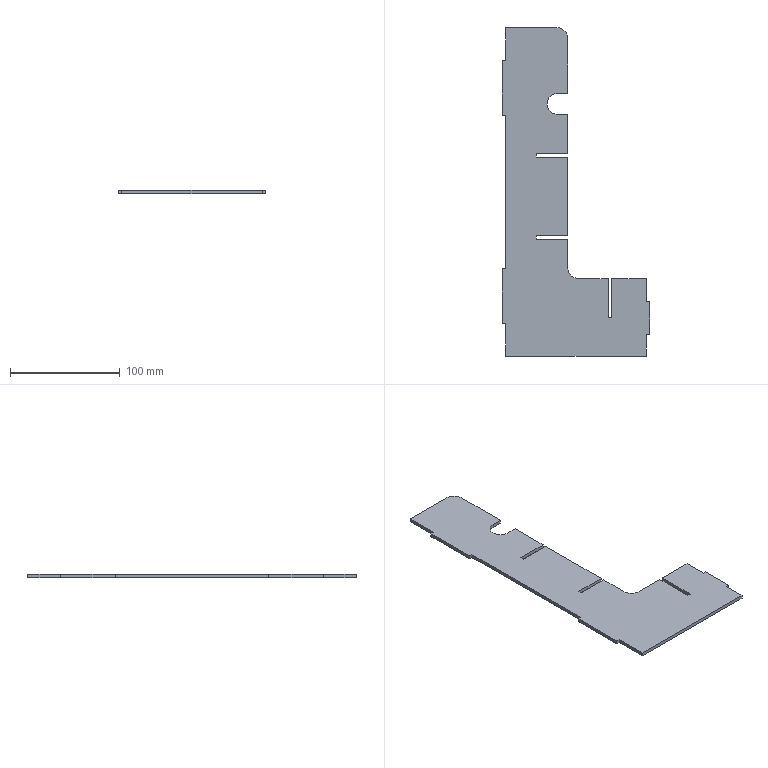Part | SolidWorks | features FlatPattern 1, SMBaseFlange 1, SheetMetal 1 | 1 solid | 38 faces | box 134.6 x 300 x 3.2 mm | volume 70099 mm3 | plane 35 | cylinder 3 | commonest cylinder face diameters 20 x2 19 x1
STEP:
#1=CARTESIAN_POINT('',(0.,-9.5,0.));
#2=VERTEX_POINT('',#1);
#3=CARTESIAN_POINT('',(0.,9.5,0.));
#4=VERTEX_POINT('',#3);
#5=CARTESIAN_POINT('',(0.,0.,0.));
#6=DIRECTION('',(0.,0.,-1.));
#7=DIRECTION('',(1.,0.,0.));
#8=AXIS2_PLACEMENT_3D('',#5,#6,#7);
#9=CIRCLE('',#8,9.5);
#10=EDGE_CURVE('',#2,#4,#9,.T.);
#11=ORIENTED_EDGE('',*,*,#10,.F.);
#12=CARTESIAN_POINT('',(0.,-9.5,-3.2));
#13=VERTEX_POINT('',#12);
#14=CARTESIAN_POINT('',(0.,-9.5,-3.2));
#15=DIRECTION('',(0.,0.,1.));
#16=VECTOR('',#15,1000.);
#17=LINE('',#14,#16);
#18=EDGE_CURVE('',#13,#2,#17,.T.);
#19=ORIENTED_EDGE('',*,*,#18,.F.);
#20=CARTESIAN_POINT('',(0.,9.5,-3.2));
#21=VERTEX_POINT('',#20);
#22=CARTESIAN_POINT('',(0.,0.,-3.2));
#23=DIRECTION('',(0.,0.,-1.));
#24=DIRECTION('',(1.,0.,0.));
#25=AXIS2_PLACEMENT_3D('',#22,#23,#24);
#26=CIRCLE('',#25,9.5);
#27=EDGE_CURVE('',#13,#21,#26,.T.);
#28=ORIENTED_EDGE('',*,*,#27,.T.);
#29=CARTESIAN_POINT('',(0.,9.5,-3.2));
#30=DIRECTION('',(0.,0.,1.));
#31=VECTOR('',#30,1000.);
#32=LINE('',#29,#31);
#33=EDGE_CURVE('',#21,#4,#32,.T.);
#34=ORIENTED_EDGE('',*,*,#33,.T.);
#35=EDGE_LOOP('',(#11,#19,#28,#34));
#36=FACE_OUTER_BOUND('',#35,.T.);
#37=CARTESIAN_POINT('',(0.,0.,-3.2));
#38=DIRECTION('',(0.,0.,1.));
#39=DIRECTION('',(1.,0.,0.));
#40=AXIS2_PLACEMENT_3D('',#37,#38,#39);
#41=CYLINDRICAL_SURFACE('',#40,9.5);
#42=ADVANCED_FACE('',(#36),#41,.F.);
#43=CARTESIAN_POINT('',(9.5,-9.5,0.));
#44=VERTEX_POINT('',#43);
#45=CARTESIAN_POINT('',(0.,-9.5,0.));
#46=DIRECTION('',(-1.,0.,0.));
#47=VECTOR('',#46,1000.);
#48=LINE('',#45,#47);
#49=EDGE_CURVE('',#44,#2,#48,.T.);
#50=ORIENTED_EDGE('',*,*,#49,.F.);
#51=CARTESIAN_POINT('',(9.5,-9.5,-3.2));
#52=VERTEX_POINT('',#51);
#53=CARTESIAN_POINT('',(9.5,-9.5,-3.2));
#54=DIRECTION('',(0.,0.,1.));
#55=VECTOR('',#54,1000.);
#56=LINE('',#53,#55);
#57=EDGE_CURVE('',#52,#44,#56,.T.);
#58=ORIENTED_EDGE('',*,*,#57,.F.);
#59=CARTESIAN_POINT('',(0.,-9.5,-3.2));
#60=DIRECTION('',(-1.,0.,0.));
#61=VECTOR('',#60,1000.);
#62=LINE('',#59,#61);
#63=EDGE_CURVE('',#52,#13,#62,.T.);
#64=ORIENTED_EDGE('',*,*,#63,.T.);
#65=ORIENTED_EDGE('',*,*,#18,.T.);
#66=EDGE_LOOP('',(#50,#58,#64,#65));
#67=FACE_OUTER_BOUND('',#66,.T.);
#68=CARTESIAN_POINT('',(0.,-9.5,-3.2));
#69=DIRECTION('',(0.,1.,0.));
#70=DIRECTION('',(0.,0.,1.));
#71=AXIS2_PLACEMENT_3D('',#68,#69,#70);
#72=PLANE('',#71);
#73=ADVANCED_FACE('',(#67),#72,.T.);
#74=CARTESIAN_POINT('',(9.5,-45.5,0.));
#75=VERTEX_POINT('',#74);
#76=CARTESIAN_POINT('',(9.5,-9.5,0.));
#77=DIRECTION('',(0.,1.,0.));
#78=VECTOR('',#77,1000.);
#79=LINE('',#76,#78);
#80=EDGE_CURVE('',#75,#44,#79,.T.);
#81=ORIENTED_EDGE('',*,*,#80,.F.);
#82=CARTESIAN_POINT('',(9.5,-45.5,-3.2));
#83=VERTEX_POINT('',#82);
#84=CARTESIAN_POINT('',(9.5,-45.5,-3.2));
#85=DIRECTION('',(0.,0.,1.));
#86=VECTOR('',#85,1000.);
#87=LINE('',#84,#86);
#88=EDGE_CURVE('',#83,#75,#87,.T.);
#89=ORIENTED_EDGE('',*,*,#88,.F.);
#90=CARTESIAN_POINT('',(9.5,-9.5,-3.2));
#91=DIRECTION('',(0.,1.,0.));
#92=VECTOR('',#91,1000.);
#93=LINE('',#90,#92);
#94=EDGE_CURVE('',#83,#52,#93,.T.);
#95=ORIENTED_EDGE('',*,*,#94,.T.);
#96=ORIENTED_EDGE('',*,*,#57,.T.);
#97=EDGE_LOOP('',(#81,#89,#95,#96));
#98=FACE_OUTER_BOUND('',#97,.T.);
#99=CARTESIAN_POINT('',(9.5,-9.5,-3.2));
#100=DIRECTION('',(1.,0.,0.));
#101=DIRECTION('',(0.,1.,0.));
#102=AXIS2_PLACEMENT_3D('',#99,#100,#101);
#103=PLANE('',#102);
#104=ADVANCED_FACE('',(#98),#103,.T.);
#105=CARTESIAN_POINT('',(-19.3,-45.5,0.));
#106=VERTEX_POINT('',#105);
#107=CARTESIAN_POINT('',(9.5,-45.5,0.));
#108=DIRECTION('',(1.,0.,0.));
#109=VECTOR('',#108,1000.);
#110=LINE('',#107,#109);
#111=EDGE_CURVE('',#106,#75,#110,.T.);
#112=ORIENTED_EDGE('',*,*,#111,.F.);
#113=CARTESIAN_POINT('',(-19.3,-45.5,-3.2));
#114=VERTEX_POINT('',#113);
#115=CARTESIAN_POINT('',(-19.3,-45.5,-3.2));
#116=DIRECTION('',(0.,0.,1.));
#117=VECTOR('',#116,1000.);
#118=LINE('',#115,#117);
#119=EDGE_CURVE('',#114,#106,#118,.T.);
#120=ORIENTED_EDGE('',*,*,#119,.F.);
#121=CARTESIAN_POINT('',(9.5,-45.5,-3.2));
#122=DIRECTION('',(1.,0.,0.));
#123=VECTOR('',#122,1000.);
#124=LINE('',#121,#123);
#125=EDGE_CURVE('',#114,#83,#124,.T.);
#126=ORIENTED_EDGE('',*,*,#125,.T.);
#127=ORIENTED_EDGE('',*,*,#88,.T.);
#128=EDGE_LOOP('',(#112,#120,#126,#127));
#129=FACE_OUTER_BOUND('',#128,.T.);
#130=CARTESIAN_POINT('',(9.5,-45.5,-3.2));
#131=DIRECTION('',(0.,-1.,0.));
#132=DIRECTION('',(0.,0.,-1.));
#133=AXIS2_PLACEMENT_3D('',#130,#131,#132);
#134=PLANE('',#133);
#135=ADVANCED_FACE('',(#129),#134,.T.);
#136=CARTESIAN_POINT('',(-19.3,-48.7,0.));
#137=VERTEX_POINT('',#136);
#138=CARTESIAN_POINT('',(-19.3,-45.5,0.));
#139=DIRECTION('',(0.,1.,0.));
#140=VECTOR('',#139,1000.);
#141=LINE('',#138,#140);
#142=EDGE_CURVE('',#137,#106,#141,.T.);
#143=ORIENTED_EDGE('',*,*,#142,.F.);
#144=CARTESIAN_POINT('',(-19.3,-48.7,-3.2));
#145=VERTEX_POINT('',#144);
#146=CARTESIAN_POINT('',(-19.3,-48.7,-3.2));
#147=DIRECTION('',(0.,0.,1.));
#148=VECTOR('',#147,1000.);
#149=LINE('',#146,#148);
#150=EDGE_CURVE('',#145,#137,#149,.T.);
#151=ORIENTED_EDGE('',*,*,#150,.F.);
#152=CARTESIAN_POINT('',(-19.3,-45.5,-3.2));
#153=DIRECTION('',(0.,1.,0.));
#154=VECTOR('',#153,1000.);
#155=LINE('',#152,#154);
#156=EDGE_CURVE('',#145,#114,#155,.T.);
#157=ORIENTED_EDGE('',*,*,#156,.T.);
#158=ORIENTED_EDGE('',*,*,#119,.T.);
#159=EDGE_LOOP('',(#143,#151,#157,#158));
#160=FACE_OUTER_BOUND('',#159,.T.);
#161=CARTESIAN_POINT('',(-19.3,-45.5,-3.2));
#162=DIRECTION('',(1.,0.,0.));
#163=DIRECTION('',(0.,0.,-1.));
#164=AXIS2_PLACEMENT_3D('',#161,#162,#163);
#165=PLANE('',#164);
#166=ADVANCED_FACE('',(#160),#165,.T.);
#167=CARTESIAN_POINT('',(9.5,-48.7,0.));
#168=VERTEX_POINT('',#167);
#169=CARTESIAN_POINT('',(-19.3,-48.7,0.));
#170=DIRECTION('',(-1.,0.,0.));
#171=VECTOR('',#170,1000.);
#172=LINE('',#169,#171);
#173=EDGE_CURVE('',#168,#137,#172,.T.);
#174=ORIENTED_EDGE('',*,*,#173,.F.);
#175=CARTESIAN_POINT('',(9.5,-48.7,-3.2));
#176=VERTEX_POINT('',#175);
#177=CARTESIAN_POINT('',(9.5,-48.7,-3.2));
#178=DIRECTION('',(0.,0.,1.));
#179=VECTOR('',#178,1000.);
#180=LINE('',#177,#179);
#181=EDGE_CURVE('',#176,#168,#180,.T.);
#182=ORIENTED_EDGE('',*,*,#181,.F.);
#183=CARTESIAN_POINT('',(-19.3,-48.7,-3.2));
#184=DIRECTION('',(-1.,0.,0.));
#185=VECTOR('',#184,1000.);
#186=LINE('',#183,#185);
#187=EDGE_CURVE('',#176,#145,#186,.T.);
#188=ORIENTED_EDGE('',*,*,#187,.T.);
#189=ORIENTED_EDGE('',*,*,#150,.T.);
#190=EDGE_LOOP('',(#174,#182,#188,#189));
#191=FACE_OUTER_BOUND('',#190,.T.);
#192=CARTESIAN_POINT('',(-19.3,-48.7,-3.2));
#193=DIRECTION('',(0.,1.,0.));
#194=DIRECTION('',(0.,0.,1.));
#195=AXIS2_PLACEMENT_3D('',#192,#193,#194);
#196=PLANE('',#195);
#197=ADVANCED_FACE('',(#191),#196,.T.);
#198=CARTESIAN_POINT('',(9.5,-120.5,0.));
#199=VERTEX_POINT('',#198);
#200=CARTESIAN_POINT('',(9.5,-48.7,0.));
#201=DIRECTION('',(0.,1.,0.));
#202=VECTOR('',#201,1000.);
#203=LINE('',#200,#202);
#204=EDGE_CURVE('',#199,#168,#203,.T.);
#205=ORIENTED_EDGE('',*,*,#204,.F.);
#206=CARTESIAN_POINT('',(9.5,-120.5,-3.2));
#207=VERTEX_POINT('',#206);
#208=CARTESIAN_POINT('',(9.5,-120.5,-3.2));
#209=DIRECTION('',(0.,0.,1.));
#210=VECTOR('',#209,1000.);
#211=LINE('',#208,#210);
#212=EDGE_CURVE('',#207,#199,#211,.T.);
#213=ORIENTED_EDGE('',*,*,#212,.F.);
#214=CARTESIAN_POINT('',(9.5,-48.7,-3.2));
#215=DIRECTION('',(0.,1.,0.));
#216=VECTOR('',#215,1000.);
#217=LINE('',#214,#216);
#218=EDGE_CURVE('',#207,#176,#217,.T.);
#219=ORIENTED_EDGE('',*,*,#218,.T.);
#220=ORIENTED_EDGE('',*,*,#181,.T.);
#221=EDGE_LOOP('',(#205,#213,#219,#220));
#222=FACE_OUTER_BOUND('',#221,.T.);
#223=CARTESIAN_POINT('',(9.5,-48.7,-3.2));
#224=DIRECTION('',(1.,0.,0.));
#225=DIRECTION('',(0.,1.,0.));
#226=AXIS2_PLACEMENT_3D('',#223,#224,#225);
#227=PLANE('',#226);
#228=ADVANCED_FACE('',(#222),#227,.T.);
#229=CARTESIAN_POINT('',(-19.3,-120.5,0.));
#230=VERTEX_POINT('',#229);
#231=CARTESIAN_POINT('',(9.5,-120.5,0.));
#232=DIRECTION('',(1.,0.,0.));
#233=VECTOR('',#232,1000.);
#234=LINE('',#231,#233);
#235=EDGE_CURVE('',#230,#199,#234,.T.);
#236=ORIENTED_EDGE('',*,*,#235,.F.);
#237=CARTESIAN_POINT('',(-19.3,-120.5,-3.2));
#238=VERTEX_POINT('',#237);
#239=CARTESIAN_POINT('',(-19.3,-120.5,-3.2));
#240=DIRECTION('',(0.,0.,1.));
#241=VECTOR('',#240,1000.);
#242=LINE('',#239,#241);
#243=EDGE_CURVE('',#238,#230,#242,.T.);
#244=ORIENTED_EDGE('',*,*,#243,.F.);
#245=CARTESIAN_POINT('',(9.5,-120.5,-3.2));
#246=DIRECTION('',(1.,0.,0.));
#247=VECTOR('',#246,1000.);
#248=LINE('',#245,#247);
#249=EDGE_CURVE('',#238,#207,#248,.T.);
#250=ORIENTED_EDGE('',*,*,#249,.T.);
#251=ORIENTED_EDGE('',*,*,#212,.T.);
#252=EDGE_LOOP('',(#236,#244,#250,#251));
#253=FACE_OUTER_BOUND('',#252,.T.);
#254=CARTESIAN_POINT('',(9.5,-120.5,-3.2));
#255=DIRECTION('',(0.,-1.,0.));
#256=DIRECTION('',(0.,0.,-1.));
#257=AXIS2_PLACEMENT_3D('',#254,#255,#256);
#258=PLANE('',#257);
#259=ADVANCED_FACE('',(#253),#258,.T.);
#260=CARTESIAN_POINT('',(-19.3,-123.7,0.));
#261=VERTEX_POINT('',#260);
#262=CARTESIAN_POINT('',(-19.3,-120.5,0.));
#263=DIRECTION('',(0.,1.,0.));
#264=VECTOR('',#263,1000.);
#265=LINE('',#262,#264);
#266=EDGE_CURVE('',#261,#230,#265,.T.);
#267=ORIENTED_EDGE('',*,*,#266,.F.);
#268=CARTESIAN_POINT('',(-19.3,-123.7,-3.2));
#269=VERTEX_POINT('',#268);
#270=CARTESIAN_POINT('',(-19.3,-123.7,-3.2));
#271=DIRECTION('',(0.,0.,1.));
#272=VECTOR('',#271,1000.);
#273=LINE('',#270,#272);
#274=EDGE_CURVE('',#269,#261,#273,.T.);
#275=ORIENTED_EDGE('',*,*,#274,.F.);
#276=CARTESIAN_POINT('',(-19.3,-120.5,-3.2));
#277=DIRECTION('',(0.,1.,0.));
#278=VECTOR('',#277,1000.);
#279=LINE('',#276,#278);
#280=EDGE_CURVE('',#269,#238,#279,.T.);
#281=ORIENTED_EDGE('',*,*,#280,.T.);
#282=ORIENTED_EDGE('',*,*,#243,.T.);
#283=EDGE_LOOP('',(#267,#275,#281,#282));
#284=FACE_OUTER_BOUND('',#283,.T.);
#285=CARTESIAN_POINT('',(-19.3,-120.5,-3.2));
#286=DIRECTION('',(1.,0.,0.));
#287=DIRECTION('',(0.,1.,0.));
#288=AXIS2_PLACEMENT_3D('',#285,#286,#287);
#289=PLANE('',#288);
#290=ADVANCED_FACE('',(#284),#289,.T.);
#291=CARTESIAN_POINT('',(9.5,-123.7,0.));
#292=VERTEX_POINT('',#291);
#293=CARTESIAN_POINT('',(-19.3,-123.7,0.));
#294=DIRECTION('',(-1.,0.,0.));
#295=VECTOR('',#294,1000.);
#296=LINE('',#293,#295);
#297=EDGE_CURVE('',#292,#261,#296,.T.);
#298=ORIENTED_EDGE('',*,*,#297,.F.);
#299=CARTESIAN_POINT('',(9.5,-123.7,-3.2));
#300=VERTEX_POINT('',#299);
#301=CARTESIAN_POINT('',(9.5,-123.7,-3.2));
#302=DIRECTION('',(0.,0.,1.));
#303=VECTOR('',#302,1000.);
#304=LINE('',#301,#303);
#305=EDGE_CURVE('',#300,#292,#304,.T.);
#306=ORIENTED_EDGE('',*,*,#305,.F.);
#307=CARTESIAN_POINT('',(-19.3,-123.7,-3.2));
#308=DIRECTION('',(-1.,0.,0.));
#309=VECTOR('',#308,1000.);
#310=LINE('',#307,#309);
#311=EDGE_CURVE('',#300,#269,#310,.T.);
#312=ORIENTED_EDGE('',*,*,#311,.T.);
#313=ORIENTED_EDGE('',*,*,#274,.T.);
#314=EDGE_LOOP('',(#298,#306,#312,#313));
#315=FACE_OUTER_BOUND('',#314,.T.);
#316=CARTESIAN_POINT('',(-19.3,-123.7,-3.2));
#317=DIRECTION('',(0.,1.,0.));
#318=DIRECTION('',(0.,0.,1.));
#319=AXIS2_PLACEMENT_3D('',#316,#317,#318);
#320=PLANE('',#319);
#321=ADVANCED_FACE('',(#315),#320,.T.);
#322=CARTESIAN_POINT('',(9.5,-149.5,0.));
#323=VERTEX_POINT('',#322);
#324=CARTESIAN_POINT('',(9.5,-123.7,0.));
#325=DIRECTION('',(0.,1.,0.));
#326=VECTOR('',#325,1000.);
#327=LINE('',#324,#326);
#328=EDGE_CURVE('',#323,#292,#327,.T.);
#329=ORIENTED_EDGE('',*,*,#328,.F.);
#330=CARTESIAN_POINT('',(9.5,-149.5,-3.2));
#331=VERTEX_POINT('',#330);
#332=CARTESIAN_POINT('',(9.5,-149.5,-3.2));
#333=DIRECTION('',(0.,0.,1.));
#334=VECTOR('',#333,1000.);
#335=LINE('',#332,#334);
#336=EDGE_CURVE('',#331,#323,#335,.T.);
#337=ORIENTED_EDGE('',*,*,#336,.F.);
#338=CARTESIAN_POINT('',(9.5,-123.7,-3.2));
#339=DIRECTION('',(0.,1.,0.));
#340=VECTOR('',#339,1000.);
#341=LINE('',#338,#340);
#342=EDGE_CURVE('',#331,#300,#341,.T.);
#343=ORIENTED_EDGE('',*,*,#342,.T.);
#344=ORIENTED_EDGE('',*,*,#305,.T.);
#345=EDGE_LOOP('',(#329,#337,#343,#344));
#346=FACE_OUTER_BOUND('',#345,.T.);
#347=CARTESIAN_POINT('',(9.5,-123.7,-3.2));
#348=DIRECTION('',(1.,0.,0.));
#349=DIRECTION('',(0.,1.,0.));
#350=AXIS2_PLACEMENT_3D('',#347,#348,#349);
#351=PLANE('',#350);
#352=ADVANCED_FACE('',(#346),#351,.T.);
#353=CARTESIAN_POINT('',(19.5,-159.5,0.));
#354=VERTEX_POINT('',#353);
#355=CARTESIAN_POINT('',(19.5,-149.5,0.));
#356=DIRECTION('',(0.,0.,-1.));
#357=DIRECTION('',(-1.,0.,0.));
#358=AXIS2_PLACEMENT_3D('',#355,#356,#357);
#359=CIRCLE('',#358,10.);
#360=EDGE_CURVE('',#354,#323,#359,.T.);
#361=ORIENTED_EDGE('',*,*,#360,.F.);
#362=CARTESIAN_POINT('',(19.5,-159.5,-3.2));
#363=VERTEX_POINT('',#362);
#364=CARTESIAN_POINT('',(19.5,-159.5,-3.2));
#365=DIRECTION('',(0.,0.,1.));
#366=VECTOR('',#365,1000.);
#367=LINE('',#364,#366);
#368=EDGE_CURVE('',#363,#354,#367,.T.);
#369=ORIENTED_EDGE('',*,*,#368,.F.);
#370=CARTESIAN_POINT('',(19.5,-149.5,-3.2));
#371=DIRECTION('',(0.,0.,-1.));
#372=DIRECTION('',(-1.,0.,0.));
#373=AXIS2_PLACEMENT_3D('',#370,#371,#372);
#374=CIRCLE('',#373,10.);
#375=EDGE_CURVE('',#363,#331,#374,.T.);
#376=ORIENTED_EDGE('',*,*,#375,.T.);
#377=ORIENTED_EDGE('',*,*,#336,.T.);
#378=EDGE_LOOP('',(#361,#369,#376,#377));
#379=FACE_OUTER_BOUND('',#378,.T.);
#380=CARTESIAN_POINT('',(19.5,-149.5,-3.2));
#381=DIRECTION('',(0.,0.,1.));
#382=DIRECTION('',(1.,0.,0.));
#383=AXIS2_PLACEMENT_3D('',#380,#381,#382);
#384=CYLINDRICAL_SURFACE('',#383,10.);
#385=ADVANCED_FACE('',(#379),#384,.F.);
#386=CARTESIAN_POINT('',(46.3,-159.5,0.));
#387=VERTEX_POINT('',#386);
#388=CARTESIAN_POINT('',(46.3,-159.5,0.));
#389=DIRECTION('',(-1.,0.,0.));
#390=VECTOR('',#389,1000.);
#391=LINE('',#388,#390);
#392=EDGE_CURVE('',#387,#354,#391,.T.);
#393=ORIENTED_EDGE('',*,*,#392,.F.);
#394=CARTESIAN_POINT('',(46.3,-159.5,-3.2));
#395=VERTEX_POINT('',#394);
#396=CARTESIAN_POINT('',(46.3,-159.5,-3.2));
#397=DIRECTION('',(0.,0.,1.));
#398=VECTOR('',#397,1000.);
#399=LINE('',#396,#398);
#400=EDGE_CURVE('',#395,#387,#399,.T.);
#401=ORIENTED_EDGE('',*,*,#400,.F.);
#402=CARTESIAN_POINT('',(46.3,-159.5,-3.2));
#403=DIRECTION('',(-1.,0.,0.));
#404=VECTOR('',#403,1000.);
#405=LINE('',#402,#404);
#406=EDGE_CURVE('',#395,#363,#405,.T.);
#407=ORIENTED_EDGE('',*,*,#406,.T.);
#408=ORIENTED_EDGE('',*,*,#368,.T.);
#409=EDGE_LOOP('',(#393,#401,#407,#408));
#410=FACE_OUTER_BOUND('',#409,.T.);
#411=CARTESIAN_POINT('',(46.3,-159.5,-3.2));
#412=DIRECTION('',(0.,1.,0.));
#413=DIRECTION('',(-1.,0.,0.));
#414=AXIS2_PLACEMENT_3D('',#411,#412,#413);
#415=PLANE('',#414);
#416=ADVANCED_FACE('',(#410),#415,.T.);
#417=CARTESIAN_POINT('',(46.3,-195.5,0.));
#418=VERTEX_POINT('',#417);
#419=CARTESIAN_POINT('',(46.3,-195.5,0.));
#420=DIRECTION('',(0.,1.,0.));
#421=VECTOR('',#420,1000.);
#422=LINE('',#419,#421);
#423=EDGE_CURVE('',#418,#387,#422,.T.);
#424=ORIENTED_EDGE('',*,*,#423,.F.);
#425=CARTESIAN_POINT('',(46.3,-195.5,-3.2));
#426=VERTEX_POINT('',#425);
#427=CARTESIAN_POINT('',(46.3,-195.5,-3.2));
#428=DIRECTION('',(0.,0.,1.));
#429=VECTOR('',#428,1000.);
#430=LINE('',#427,#429);
#431=EDGE_CURVE('',#426,#418,#430,.T.);
#432=ORIENTED_EDGE('',*,*,#431,.F.);
#433=CARTESIAN_POINT('',(46.3,-195.5,-3.2));
#434=DIRECTION('',(0.,1.,0.));
#435=VECTOR('',#434,1000.);
#436=LINE('',#433,#435);
#437=EDGE_CURVE('',#426,#395,#436,.T.);
#438=ORIENTED_EDGE('',*,*,#437,.T.);
#439=ORIENTED_EDGE('',*,*,#400,.T.);
#440=EDGE_LOOP('',(#424,#432,#438,#439));
#441=FACE_OUTER_BOUND('',#440,.T.);
#442=CARTESIAN_POINT('',(46.3,-195.5,-3.2));
#443=DIRECTION('',(1.,0.,0.));
#444=DIRECTION('',(0.,1.,0.));
#445=AXIS2_PLACEMENT_3D('',#442,#443,#444);
#446=PLANE('',#445);
#447=ADVANCED_FACE('',(#441),#446,.T.);
#448=CARTESIAN_POINT('',(49.5,-195.5,0.));
#449=VERTEX_POINT('',#448);
#450=CARTESIAN_POINT('',(49.5,-195.5,0.));
#451=DIRECTION('',(-1.,0.,0.));
#452=VECTOR('',#451,1000.);
#453=LINE('',#450,#452);
#454=EDGE_CURVE('',#449,#418,#453,.T.);
#455=ORIENTED_EDGE('',*,*,#454,.F.);
#456=CARTESIAN_POINT('',(49.5,-195.5,-3.2));
#457=VERTEX_POINT('',#456);
#458=CARTESIAN_POINT('',(49.5,-195.5,-3.2));
#459=DIRECTION('',(0.,0.,1.));
#460=VECTOR('',#459,1000.);
#461=LINE('',#458,#460);
#462=EDGE_CURVE('',#457,#449,#461,.T.);
#463=ORIENTED_EDGE('',*,*,#462,.F.);
#464=CARTESIAN_POINT('',(49.5,-195.5,-3.2));
#465=DIRECTION('',(-1.,0.,0.));
#466=VECTOR('',#465,1000.);
#467=LINE('',#464,#466);
#468=EDGE_CURVE('',#457,#426,#467,.T.);
#469=ORIENTED_EDGE('',*,*,#468,.T.);
#470=ORIENTED_EDGE('',*,*,#431,.T.);
#471=EDGE_LOOP('',(#455,#463,#469,#470));
#472=FACE_OUTER_BOUND('',#471,.T.);
#473=CARTESIAN_POINT('',(49.5,-195.5,-3.2));
#474=DIRECTION('',(0.,1.,0.));
#475=DIRECTION('',(0.,0.,1.));
#476=AXIS2_PLACEMENT_3D('',#473,#474,#475);
#477=PLANE('',#476);
#478=ADVANCED_FACE('',(#472),#477,.T.);
#479=CARTESIAN_POINT('',(49.5,-159.5,0.));
#480=VERTEX_POINT('',#479);
#481=CARTESIAN_POINT('',(49.5,-159.5,0.));
#482=DIRECTION('',(0.,-1.,0.));
#483=VECTOR('',#482,1000.);
#484=LINE('',#481,#483);
#485=EDGE_CURVE('',#480,#449,#484,.T.);
#486=ORIENTED_EDGE('',*,*,#485,.F.);
#487=CARTESIAN_POINT('',(49.5,-159.5,-3.2));
#488=VERTEX_POINT('',#487);
#489=CARTESIAN_POINT('',(49.5,-159.5,-3.2));
#490=DIRECTION('',(0.,0.,1.));
#491=VECTOR('',#490,1000.);
#492=LINE('',#489,#491);
#493=EDGE_CURVE('',#488,#480,#492,.T.);
#494=ORIENTED_EDGE('',*,*,#493,.F.);
#495=CARTESIAN_POINT('',(49.5,-159.5,-3.2));
#496=DIRECTION('',(0.,-1.,0.));
#497=VECTOR('',#496,1000.);
#498=LINE('',#495,#497);
#499=EDGE_CURVE('',#488,#457,#498,.T.);
#500=ORIENTED_EDGE('',*,*,#499,.T.);
#501=ORIENTED_EDGE('',*,*,#462,.T.);
#502=EDGE_LOOP('',(#486,#494,#500,#501));
#503=FACE_OUTER_BOUND('',#502,.T.);
#504=CARTESIAN_POINT('',(49.5,-159.5,-3.2));
#505=DIRECTION('',(-1.,0.,0.));
#506=DIRECTION('',(0.,-1.,0.));
#507=AXIS2_PLACEMENT_3D('',#504,#505,#506);
#508=PLANE('',#507);
#509=ADVANCED_FACE('',(#503),#508,.T.);
#510=CARTESIAN_POINT('',(81.3,-159.5,0.));
#511=VERTEX_POINT('',#510);
#512=CARTESIAN_POINT('',(81.3,-159.5,0.));
#513=DIRECTION('',(-1.,0.,0.));
#514=VECTOR('',#513,1000.);
#515=LINE('',#512,#514);
#516=EDGE_CURVE('',#511,#480,#515,.T.);
#517=ORIENTED_EDGE('',*,*,#516,.F.);
#518=CARTESIAN_POINT('',(81.3,-159.5,-3.2));
#519=VERTEX_POINT('',#518);
#520=CARTESIAN_POINT('',(81.3,-159.5,-3.2));
#521=DIRECTION('',(0.,0.,1.));
#522=VECTOR('',#521,1000.);
#523=LINE('',#520,#522);
#524=EDGE_CURVE('',#519,#511,#523,.T.);
#525=ORIENTED_EDGE('',*,*,#524,.F.);
#526=CARTESIAN_POINT('',(81.3,-159.5,-3.2));
#527=DIRECTION('',(-1.,0.,0.));
#528=VECTOR('',#527,1000.);
#529=LINE('',#526,#528);
#530=EDGE_CURVE('',#519,#488,#529,.T.);
#531=ORIENTED_EDGE('',*,*,#530,.T.);
#532=ORIENTED_EDGE('',*,*,#493,.T.);
#533=EDGE_LOOP('',(#517,#525,#531,#532));
#534=FACE_OUTER_BOUND('',#533,.T.);
#535=CARTESIAN_POINT('',(81.3,-159.5,-3.2));
#536=DIRECTION('',(0.,1.,0.));
#537=DIRECTION('',(-1.,0.,0.));
#538=AXIS2_PLACEMENT_3D('',#535,#536,#537);
#539=PLANE('',#538);
#540=ADVANCED_FACE('',(#534),#539,.T.);
#541=CARTESIAN_POINT('',(81.3,-180.5,0.));
#542=VERTEX_POINT('',#541);
#543=CARTESIAN_POINT('',(81.3,-180.5,0.));
#544=DIRECTION('',(0.,1.,0.));
#545=VECTOR('',#544,1000.);
#546=LINE('',#543,#545);
#547=EDGE_CURVE('',#542,#511,#546,.T.);
#548=ORIENTED_EDGE('',*,*,#547,.F.);
#549=CARTESIAN_POINT('',(81.3,-180.5,-3.2));
#550=VERTEX_POINT('',#549);
#551=CARTESIAN_POINT('',(81.3,-180.5,-3.2));
#552=DIRECTION('',(0.,0.,1.));
#553=VECTOR('',#552,1000.);
#554=LINE('',#551,#553);
#555=EDGE_CURVE('',#550,#542,#554,.T.);
#556=ORIENTED_EDGE('',*,*,#555,.F.);
#557=CARTESIAN_POINT('',(81.3,-180.5,-3.2));
#558=DIRECTION('',(0.,1.,0.));
#559=VECTOR('',#558,1000.);
#560=LINE('',#557,#559);
#561=EDGE_CURVE('',#550,#519,#560,.T.);
#562=ORIENTED_EDGE('',*,*,#561,.T.);
#563=ORIENTED_EDGE('',*,*,#524,.T.);
#564=EDGE_LOOP('',(#548,#556,#562,#563));
#565=FACE_OUTER_BOUND('',#564,.T.);
#566=CARTESIAN_POINT('',(81.3,-180.5,-3.2));
#567=DIRECTION('',(1.,0.,0.));
#568=DIRECTION('',(0.,0.,-1.));
#569=AXIS2_PLACEMENT_3D('',#566,#567,#568);
#570=PLANE('',#569);
#571=ADVANCED_FACE('',(#565),#570,.T.);
#572=CARTESIAN_POINT('',(84.3,-180.5,0.));
#573=VERTEX_POINT('',#572);
#574=CARTESIAN_POINT('',(81.3,-180.5,0.));
#575=DIRECTION('',(-1.,0.,0.));
#576=VECTOR('',#575,1000.);
#577=LINE('',#574,#576);
#578=EDGE_CURVE('',#573,#542,#577,.T.);
#579=ORIENTED_EDGE('',*,*,#578,.F.);
#580=CARTESIAN_POINT('',(84.3,-180.5,-3.2));
#581=VERTEX_POINT('',#580);
#582=CARTESIAN_POINT('',(84.3,-180.5,-3.2));
#583=DIRECTION('',(0.,0.,1.));
#584=VECTOR('',#583,1000.);
#585=LINE('',#582,#584);
#586=EDGE_CURVE('',#581,#573,#585,.T.);
#587=ORIENTED_EDGE('',*,*,#586,.F.);
#588=CARTESIAN_POINT('',(81.3,-180.5,-3.2));
#589=DIRECTION('',(-1.,0.,0.));
#590=VECTOR('',#589,1000.);
#591=LINE('',#588,#590);
#592=EDGE_CURVE('',#581,#550,#591,.T.);
#593=ORIENTED_EDGE('',*,*,#592,.T.);
#594=ORIENTED_EDGE('',*,*,#555,.T.);
#595=EDGE_LOOP('',(#579,#587,#593,#594));
#596=FACE_OUTER_BOUND('',#595,.T.);
#597=CARTESIAN_POINT('',(81.3,-180.5,-3.2));
#598=DIRECTION('',(0.,1.,0.));
#599=DIRECTION('',(0.,0.,1.));
#600=AXIS2_PLACEMENT_3D('',#597,#598,#599);
#601=PLANE('',#600);
#602=ADVANCED_FACE('',(#596),#601,.T.);
#603=CARTESIAN_POINT('',(84.3,-210.5,0.));
#604=VERTEX_POINT('',#603);
#605=CARTESIAN_POINT('',(84.3,-180.5,0.));
#606=DIRECTION('',(0.,1.,0.));
#607=VECTOR('',#606,1000.);
#608=LINE('',#605,#607);
#609=EDGE_CURVE('',#604,#573,#608,.T.);
#610=ORIENTED_EDGE('',*,*,#609,.F.);
#611=CARTESIAN_POINT('',(84.3,-210.5,-3.2));
#612=VERTEX_POINT('',#611);
#613=CARTESIAN_POINT('',(84.3,-210.5,-3.2));
#614=DIRECTION('',(0.,0.,1.));
#615=VECTOR('',#614,1000.);
#616=LINE('',#613,#615);
#617=EDGE_CURVE('',#612,#604,#616,.T.);
#618=ORIENTED_EDGE('',*,*,#617,.F.);
#619=CARTESIAN_POINT('',(84.3,-180.5,-3.2));
#620=DIRECTION('',(0.,1.,0.));
#621=VECTOR('',#620,1000.);
#622=LINE('',#619,#621);
#623=EDGE_CURVE('',#612,#581,#622,.T.);
#624=ORIENTED_EDGE('',*,*,#623,.T.);
#625=ORIENTED_EDGE('',*,*,#586,.T.);
#626=EDGE_LOOP('',(#610,#618,#624,#625));
#627=FACE_OUTER_BOUND('',#626,.T.);
#628=CARTESIAN_POINT('',(84.3,-180.5,-3.2));
#629=DIRECTION('',(1.,0.,0.));
#630=DIRECTION('',(0.,1.,0.));
#631=AXIS2_PLACEMENT_3D('',#628,#629,#630);
#632=PLANE('',#631);
#633=ADVANCED_FACE('',(#627),#632,.T.);
#634=CARTESIAN_POINT('',(81.3,-210.5,0.));
#635=VERTEX_POINT('',#634);
#636=CARTESIAN_POINT('',(84.3,-210.5,0.));
#637=DIRECTION('',(1.,0.,0.));
#638=VECTOR('',#637,1000.);
#639=LINE('',#636,#638);
#640=EDGE_CURVE('',#635,#604,#639,.T.);
#641=ORIENTED_EDGE('',*,*,#640,.F.);
#642=CARTESIAN_POINT('',(81.3,-210.5,-3.2));
#643=VERTEX_POINT('',#642);
#644=CARTESIAN_POINT('',(81.3,-210.5,-3.2));
#645=DIRECTION('',(0.,0.,1.));
#646=VECTOR('',#645,1000.);
#647=LINE('',#644,#646);
#648=EDGE_CURVE('',#643,#635,#647,.T.);
#649=ORIENTED_EDGE('',*,*,#648,.F.);
#650=CARTESIAN_POINT('',(84.3,-210.5,-3.2));
#651=DIRECTION('',(1.,0.,0.));
#652=VECTOR('',#651,1000.);
#653=LINE('',#650,#652);
#654=EDGE_CURVE('',#643,#612,#653,.T.);
#655=ORIENTED_EDGE('',*,*,#654,.T.);
#656=ORIENTED_EDGE('',*,*,#617,.T.);
#657=EDGE_LOOP('',(#641,#649,#655,#656));
#658=FACE_OUTER_BOUND('',#657,.T.);
#659=CARTESIAN_POINT('',(84.3,-210.5,-3.2));
#660=DIRECTION('',(0.,-1.,0.));
#661=DIRECTION('',(1.,0.,0.));
#662=AXIS2_PLACEMENT_3D('',#659,#660,#661);
#663=PLANE('',#662);
#664=ADVANCED_FACE('',(#658),#663,.T.);
#665=CARTESIAN_POINT('',(81.3,-230.5,0.));
#666=VERTEX_POINT('',#665);
#667=CARTESIAN_POINT('',(81.3,-230.5,0.));
#668=DIRECTION('',(0.,1.,0.));
#669=VECTOR('',#668,1000.);
#670=LINE('',#667,#669);
#671=EDGE_CURVE('',#666,#635,#670,.T.);
#672=ORIENTED_EDGE('',*,*,#671,.F.);
#673=CARTESIAN_POINT('',(81.3,-230.5,-3.2));
#674=VERTEX_POINT('',#673);
#675=CARTESIAN_POINT('',(81.3,-230.5,-3.2));
#676=DIRECTION('',(0.,0.,1.));
#677=VECTOR('',#676,1000.);
#678=LINE('',#675,#677);
#679=EDGE_CURVE('',#674,#666,#678,.T.);
#680=ORIENTED_EDGE('',*,*,#679,.F.);
#681=CARTESIAN_POINT('',(81.3,-230.5,-3.2));
#682=DIRECTION('',(0.,1.,0.));
#683=VECTOR('',#682,1000.);
#684=LINE('',#681,#683);
#685=EDGE_CURVE('',#674,#643,#684,.T.);
#686=ORIENTED_EDGE('',*,*,#685,.T.);
#687=ORIENTED_EDGE('',*,*,#648,.T.);
#688=EDGE_LOOP('',(#672,#680,#686,#687));
#689=FACE_OUTER_BOUND('',#688,.T.);
#690=CARTESIAN_POINT('',(81.3,-230.5,-3.2));
#691=DIRECTION('',(1.,0.,0.));
#692=DIRECTION('',(0.,0.,-1.));
#693=AXIS2_PLACEMENT_3D('',#690,#691,#692);
#694=PLANE('',#693);
#695=ADVANCED_FACE('',(#689),#694,.T.);
#696=CARTESIAN_POINT('',(-47.3,-230.5,0.));
#697=VERTEX_POINT('',#696);
#698=CARTESIAN_POINT('',(-47.3,-230.5,0.));
#699=DIRECTION('',(1.,0.,0.));
#700=VECTOR('',#699,1000.);
#701=LINE('',#698,#700);
#702=EDGE_CURVE('',#697,#666,#701,.T.);
#703=ORIENTED_EDGE('',*,*,#702,.F.);
#704=CARTESIAN_POINT('',(-47.3,-230.5,-3.2));
#705=VERTEX_POINT('',#704);
#706=CARTESIAN_POINT('',(-47.3,-230.5,-3.2));
#707=DIRECTION('',(0.,0.,1.));
#708=VECTOR('',#707,1000.);
#709=LINE('',#706,#708);
#710=EDGE_CURVE('',#705,#697,#709,.T.);
#711=ORIENTED_EDGE('',*,*,#710,.F.);
#712=CARTESIAN_POINT('',(-47.3,-230.5,-3.2));
#713=DIRECTION('',(1.,0.,0.));
#714=VECTOR('',#713,1000.);
#715=LINE('',#712,#714);
#716=EDGE_CURVE('',#705,#674,#715,.T.);
#717=ORIENTED_EDGE('',*,*,#716,.T.);
#718=ORIENTED_EDGE('',*,*,#679,.T.);
#719=EDGE_LOOP('',(#703,#711,#717,#718));
#720=FACE_OUTER_BOUND('',#719,.T.);
#721=CARTESIAN_POINT('',(-47.3,-230.5,-3.2));
#722=DIRECTION('',(0.,-1.,0.));
#723=DIRECTION('',(0.,0.,-1.));
#724=AXIS2_PLACEMENT_3D('',#721,#722,#723);
#725=PLANE('',#724);
#726=ADVANCED_FACE('',(#720),#725,.T.);
#727=CARTESIAN_POINT('',(-47.3,-200.5,0.));
#728=VERTEX_POINT('',#727);
#729=CARTESIAN_POINT('',(-47.3,-200.5,0.));
#730=DIRECTION('',(0.,-1.,0.));
#731=VECTOR('',#730,1000.);
#732=LINE('',#729,#731);
#733=EDGE_CURVE('',#728,#697,#732,.T.);
#734=ORIENTED_EDGE('',*,*,#733,.F.);
#735=CARTESIAN_POINT('',(-47.3,-200.5,-3.2));
#736=VERTEX_POINT('',#735);
#737=CARTESIAN_POINT('',(-47.3,-200.5,-3.2));
#738=DIRECTION('',(0.,0.,1.));
#739=VECTOR('',#738,1000.);
#740=LINE('',#737,#739);
#741=EDGE_CURVE('',#736,#728,#740,.T.);
#742=ORIENTED_EDGE('',*,*,#741,.F.);
#743=CARTESIAN_POINT('',(-47.3,-200.5,-3.2));
#744=DIRECTION('',(0.,-1.,0.));
#745=VECTOR('',#744,1000.);
#746=LINE('',#743,#745);
#747=EDGE_CURVE('',#736,#705,#746,.T.);
#748=ORIENTED_EDGE('',*,*,#747,.T.);
#749=ORIENTED_EDGE('',*,*,#710,.T.);
#750=EDGE_LOOP('',(#734,#742,#748,#749));
#751=FACE_OUTER_BOUND('',#750,.T.);
#752=CARTESIAN_POINT('',(-47.3,-200.5,-3.2));
#753=DIRECTION('',(-1.,0.,0.));
#754=DIRECTION('',(0.,-1.,0.));
#755=AXIS2_PLACEMENT_3D('',#752,#753,#754);
#756=PLANE('',#755);
#757=ADVANCED_FACE('',(#751),#756,.T.);
#758=CARTESIAN_POINT('',(-50.3,-200.5,0.));
#759=VERTEX_POINT('',#758);
#760=CARTESIAN_POINT('',(-50.3,-200.5,0.));
#761=DIRECTION('',(1.,0.,0.));
#762=VECTOR('',#761,1000.);
#763=LINE('',#760,#762);
#764=EDGE_CURVE('',#759,#728,#763,.T.);
#765=ORIENTED_EDGE('',*,*,#764,.F.);
#766=CARTESIAN_POINT('',(-50.3,-200.5,-3.2));
#767=VERTEX_POINT('',#766);
#768=CARTESIAN_POINT('',(-50.3,-200.5,-3.2));
#769=DIRECTION('',(0.,0.,1.));
#770=VECTOR('',#769,1000.);
#771=LINE('',#768,#770);
#772=EDGE_CURVE('',#767,#759,#771,.T.);
#773=ORIENTED_EDGE('',*,*,#772,.F.);
#774=CARTESIAN_POINT('',(-50.3,-200.5,-3.2));
#775=DIRECTION('',(1.,0.,0.));
#776=VECTOR('',#775,1000.);
#777=LINE('',#774,#776);
#778=EDGE_CURVE('',#767,#736,#777,.T.);
#779=ORIENTED_EDGE('',*,*,#778,.T.);
#780=ORIENTED_EDGE('',*,*,#741,.T.);
#781=EDGE_LOOP('',(#765,#773,#779,#780));
#782=FACE_OUTER_BOUND('',#781,.T.);
#783=CARTESIAN_POINT('',(-50.3,-200.5,-3.2));
#784=DIRECTION('',(0.,-1.,0.));
#785=DIRECTION('',(0.,0.,-1.));
#786=AXIS2_PLACEMENT_3D('',#783,#784,#785);
#787=PLANE('',#786);
#788=ADVANCED_FACE('',(#782),#787,.T.);
#789=CARTESIAN_POINT('',(-50.3,-150.5,0.));
#790=VERTEX_POINT('',#789);
#791=CARTESIAN_POINT('',(-50.3,-150.5,0.));
#792=DIRECTION('',(0.,-1.,0.));
#793=VECTOR('',#792,1000.);
#794=LINE('',#791,#793);
#795=EDGE_CURVE('',#790,#759,#794,.T.);
#796=ORIENTED_EDGE('',*,*,#795,.F.);
#797=CARTESIAN_POINT('',(-50.3,-150.5,-3.2));
#798=VERTEX_POINT('',#797);
#799=CARTESIAN_POINT('',(-50.3,-150.5,-3.2));
#800=DIRECTION('',(0.,0.,1.));
#801=VECTOR('',#800,1000.);
#802=LINE('',#799,#801);
#803=EDGE_CURVE('',#798,#790,#802,.T.);
#804=ORIENTED_EDGE('',*,*,#803,.F.);
#805=CARTESIAN_POINT('',(-50.3,-150.5,-3.2));
#806=DIRECTION('',(0.,-1.,0.));
#807=VECTOR('',#806,1000.);
#808=LINE('',#805,#807);
#809=EDGE_CURVE('',#798,#767,#808,.T.);
#810=ORIENTED_EDGE('',*,*,#809,.T.);
#811=ORIENTED_EDGE('',*,*,#772,.T.);
#812=EDGE_LOOP('',(#796,#804,#810,#811));
#813=FACE_OUTER_BOUND('',#812,.T.);
#814=CARTESIAN_POINT('',(-50.3,-150.5,-3.2));
#815=DIRECTION('',(-1.,0.,0.));
#816=DIRECTION('',(0.,-1.,0.));
#817=AXIS2_PLACEMENT_3D('',#814,#815,#816);
#818=PLANE('',#817);
#819=ADVANCED_FACE('',(#813),#818,.T.);
#820=CARTESIAN_POINT('',(-47.3,-150.5,0.));
#821=VERTEX_POINT('',#820);
#822=CARTESIAN_POINT('',(-47.3,-150.5,0.));
#823=DIRECTION('',(-1.,0.,0.));
#824=VECTOR('',#823,1000.);
#825=LINE('',#822,#824);
#826=EDGE_CURVE('',#821,#790,#825,.T.);
#827=ORIENTED_EDGE('',*,*,#826,.F.);
#828=CARTESIAN_POINT('',(-47.3,-150.5,-3.2));
#829=VERTEX_POINT('',#828);
#830=CARTESIAN_POINT('',(-47.3,-150.5,-3.2));
#831=DIRECTION('',(0.,0.,1.));
#832=VECTOR('',#831,1000.);
#833=LINE('',#830,#832);
#834=EDGE_CURVE('',#829,#821,#833,.T.);
#835=ORIENTED_EDGE('',*,*,#834,.F.);
#836=CARTESIAN_POINT('',(-47.3,-150.5,-3.2));
#837=DIRECTION('',(-1.,0.,0.));
#838=VECTOR('',#837,1000.);
#839=LINE('',#836,#838);
#840=EDGE_CURVE('',#829,#798,#839,.T.);
#841=ORIENTED_EDGE('',*,*,#840,.T.);
#842=ORIENTED_EDGE('',*,*,#803,.T.);
#843=EDGE_LOOP('',(#827,#835,#841,#842));
#844=FACE_OUTER_BOUND('',#843,.T.);
#845=CARTESIAN_POINT('',(-47.3,-150.5,-3.2));
#846=DIRECTION('',(0.,1.,0.));
#847=DIRECTION('',(0.,0.,1.));
#848=AXIS2_PLACEMENT_3D('',#845,#846,#847);
#849=PLANE('',#848);
#850=ADVANCED_FACE('',(#844),#849,.T.);
#851=CARTESIAN_POINT('',(-47.3,-10.5,0.));
#852=VERTEX_POINT('',#851);
#853=CARTESIAN_POINT('',(-47.3,-10.5,0.));
#854=DIRECTION('',(0.,-1.,0.));
#855=VECTOR('',#854,1000.);
#856=LINE('',#853,#855);
#857=EDGE_CURVE('',#852,#821,#856,.T.);
#858=ORIENTED_EDGE('',*,*,#857,.F.);
#859=CARTESIAN_POINT('',(-47.3,-10.5,-3.2));
#860=VERTEX_POINT('',#859);
#861=CARTESIAN_POINT('',(-47.3,-10.5,-3.2));
#862=DIRECTION('',(0.,0.,1.));
#863=VECTOR('',#862,1000.);
#864=LINE('',#861,#863);
#865=EDGE_CURVE('',#860,#852,#864,.T.);
#866=ORIENTED_EDGE('',*,*,#865,.F.);
#867=CARTESIAN_POINT('',(-47.3,-10.5,-3.2));
#868=DIRECTION('',(0.,-1.,0.));
#869=VECTOR('',#868,1000.);
#870=LINE('',#867,#869);
#871=EDGE_CURVE('',#860,#829,#870,.T.);
#872=ORIENTED_EDGE('',*,*,#871,.T.);
#873=ORIENTED_EDGE('',*,*,#834,.T.);
#874=EDGE_LOOP('',(#858,#866,#872,#873));
#875=FACE_OUTER_BOUND('',#874,.T.);
#876=CARTESIAN_POINT('',(-47.3,-10.5,-3.2));
#877=DIRECTION('',(-1.,0.,0.));
#878=DIRECTION('',(0.,-1.,0.));
#879=AXIS2_PLACEMENT_3D('',#876,#877,#878);
#880=PLANE('',#879);
#881=ADVANCED_FACE('',(#875),#880,.T.);
#882=CARTESIAN_POINT('',(-50.3,-10.5,0.));
#883=VERTEX_POINT('',#882);
#884=CARTESIAN_POINT('',(-50.3,-10.5,0.));
#885=DIRECTION('',(1.,0.,0.));
#886=VECTOR('',#885,1000.);
#887=LINE('',#884,#886);
#888=EDGE_CURVE('',#883,#852,#887,.T.);
#889=ORIENTED_EDGE('',*,*,#888,.F.);
#890=CARTESIAN_POINT('',(-50.3,-10.5,-3.2));
#891=VERTEX_POINT('',#890);
#892=CARTESIAN_POINT('',(-50.3,-10.5,-3.2));
#893=DIRECTION('',(0.,0.,1.));
#894=VECTOR('',#893,1000.);
#895=LINE('',#892,#894);
#896=EDGE_CURVE('',#891,#883,#895,.T.);
#897=ORIENTED_EDGE('',*,*,#896,.F.);
#898=CARTESIAN_POINT('',(-50.3,-10.5,-3.2));
#899=DIRECTION('',(1.,0.,0.));
#900=VECTOR('',#899,1000.);
#901=LINE('',#898,#900);
#902=EDGE_CURVE('',#891,#860,#901,.T.);
#903=ORIENTED_EDGE('',*,*,#902,.T.);
#904=ORIENTED_EDGE('',*,*,#865,.T.);
#905=EDGE_LOOP('',(#889,#897,#903,#904));
#906=FACE_OUTER_BOUND('',#905,.T.);
#907=CARTESIAN_POINT('',(-50.3,-10.5,-3.2));
#908=DIRECTION('',(0.,-1.,0.));
#909=DIRECTION('',(0.,0.,-1.));
#910=AXIS2_PLACEMENT_3D('',#907,#908,#909);
#911=PLANE('',#910);
#912=ADVANCED_FACE('',(#906),#911,.T.);
#913=CARTESIAN_POINT('',(-50.3,39.5,0.));
#914=VERTEX_POINT('',#913);
#915=CARTESIAN_POINT('',(-50.3,39.5,0.));
#916=DIRECTION('',(0.,-1.,0.));
#917=VECTOR('',#916,1000.);
#918=LINE('',#915,#917);
#919=EDGE_CURVE('',#914,#883,#918,.T.);
#920=ORIENTED_EDGE('',*,*,#919,.F.);
#921=CARTESIAN_POINT('',(-50.3,39.5,-3.2));
#922=VERTEX_POINT('',#921);
#923=CARTESIAN_POINT('',(-50.3,39.5,-3.2));
#924=DIRECTION('',(0.,0.,1.));
#925=VECTOR('',#924,1000.);
#926=LINE('',#923,#925);
#927=EDGE_CURVE('',#922,#914,#926,.T.);
#928=ORIENTED_EDGE('',*,*,#927,.F.);
#929=CARTESIAN_POINT('',(-50.3,39.5,-3.2));
#930=DIRECTION('',(0.,-1.,0.));
#931=VECTOR('',#930,1000.);
#932=LINE('',#929,#931);
#933=EDGE_CURVE('',#922,#891,#932,.T.);
#934=ORIENTED_EDGE('',*,*,#933,.T.);
#935=ORIENTED_EDGE('',*,*,#896,.T.);
#936=EDGE_LOOP('',(#920,#928,#934,#935));
#937=FACE_OUTER_BOUND('',#936,.T.);
#938=CARTESIAN_POINT('',(-50.3,39.5,-3.2));
#939=DIRECTION('',(-1.,0.,0.));
#940=DIRECTION('',(0.,-1.,0.));
#941=AXIS2_PLACEMENT_3D('',#938,#939,#940);
#942=PLANE('',#941);
#943=ADVANCED_FACE('',(#937),#942,.T.);
#944=CARTESIAN_POINT('',(-47.3,39.5,0.));
#945=VERTEX_POINT('',#944);
#946=CARTESIAN_POINT('',(-47.3,39.5,0.));
#947=DIRECTION('',(-1.,0.,0.));
#948=VECTOR('',#947,1000.);
#949=LINE('',#946,#948);
#950=EDGE_CURVE('',#945,#914,#949,.T.);
#951=ORIENTED_EDGE('',*,*,#950,.F.);
#952=CARTESIAN_POINT('',(-47.3,39.5,-3.2));
#953=VERTEX_POINT('',#952);
#954=CARTESIAN_POINT('',(-47.3,39.5,-3.2));
#955=DIRECTION('',(0.,0.,1.));
#956=VECTOR('',#955,1000.);
#957=LINE('',#954,#956);
#958=EDGE_CURVE('',#953,#945,#957,.T.);
#959=ORIENTED_EDGE('',*,*,#958,.F.);
#960=CARTESIAN_POINT('',(-47.3,39.5,-3.2));
#961=DIRECTION('',(-1.,0.,0.));
#962=VECTOR('',#961,1000.);
#963=LINE('',#960,#962);
#964=EDGE_CURVE('',#953,#922,#963,.T.);
#965=ORIENTED_EDGE('',*,*,#964,.T.);
#966=ORIENTED_EDGE('',*,*,#927,.T.);
#967=EDGE_LOOP('',(#951,#959,#965,#966));
#968=FACE_OUTER_BOUND('',#967,.T.);
#969=CARTESIAN_POINT('',(-47.3,39.5,-3.2));
#970=DIRECTION('',(0.,1.,0.));
#971=DIRECTION('',(-1.,0.,0.));
#972=AXIS2_PLACEMENT_3D('',#969,#970,#971);
#973=PLANE('',#972);
#974=ADVANCED_FACE('',(#968),#973,.T.);
#975=CARTESIAN_POINT('',(-47.3,69.5,0.));
#976=VERTEX_POINT('',#975);
#977=CARTESIAN_POINT('',(-47.3,69.5,0.));
#978=DIRECTION('',(0.,-1.,0.));
#979=VECTOR('',#978,1000.);
#980=LINE('',#977,#979);
#981=EDGE_CURVE('',#976,#945,#980,.T.);
#982=ORIENTED_EDGE('',*,*,#981,.F.);
#983=CARTESIAN_POINT('',(-47.3,69.5,-3.2));
#984=VERTEX_POINT('',#983);
#985=CARTESIAN_POINT('',(-47.3,69.5,-3.2));
#986=DIRECTION('',(0.,0.,1.));
#987=VECTOR('',#986,1000.);
#988=LINE('',#985,#987);
#989=EDGE_CURVE('',#984,#976,#988,.T.);
#990=ORIENTED_EDGE('',*,*,#989,.F.);
#991=CARTESIAN_POINT('',(-47.3,69.5,-3.2));
#992=DIRECTION('',(0.,-1.,0.));
#993=VECTOR('',#992,1000.);
#994=LINE('',#991,#993);
#995=EDGE_CURVE('',#984,#953,#994,.T.);
#996=ORIENTED_EDGE('',*,*,#995,.T.);
#997=ORIENTED_EDGE('',*,*,#958,.T.);
#998=EDGE_LOOP('',(#982,#990,#996,#997));
#999=FACE_OUTER_BOUND('',#998,.T.);
#1000=CARTESIAN_POINT('',(-47.3,69.5,-3.2));
#1001=DIRECTION('',(-1.,0.,0.));
#1002=DIRECTION('',(0.,-1.,0.));
#1003=AXIS2_PLACEMENT_3D('',#1000,#1001,#1002);
#1004=PLANE('',#1003);
#1005=ADVANCED_FACE('',(#999),#1004,.T.);
#1006=CARTESIAN_POINT('',(-0.5,69.5,0.));
#1007=VERTEX_POINT('',#1006);
#1008=CARTESIAN_POINT('',(-0.5,69.5,0.));
#1009=DIRECTION('',(-1.,0.,0.));
#1010=VECTOR('',#1009,1000.);
#1011=LINE('',#1008,#1010);
#1012=EDGE_CURVE('',#1007,#976,#1011,.T.);
#1013=ORIENTED_EDGE('',*,*,#1012,.F.);
#1014=CARTESIAN_POINT('',(-0.5,69.5,-3.2));
#1015=VERTEX_POINT('',#1014);
#1016=CARTESIAN_POINT('',(-0.5,69.5,-3.2));
#1017=DIRECTION('',(0.,0.,1.));
#1018=VECTOR('',#1017,1000.);
#1019=LINE('',#1016,#1018);
#1020=EDGE_CURVE('',#1015,#1007,#1019,.T.);
#1021=ORIENTED_EDGE('',*,*,#1020,.F.);
#1022=CARTESIAN_POINT('',(-0.5,69.5,-3.2));
#1023=DIRECTION('',(-1.,0.,0.));
#1024=VECTOR('',#1023,1000.);
#1025=LINE('',#1022,#1024);
#1026=EDGE_CURVE('',#1015,#984,#1025,.T.);
#1027=ORIENTED_EDGE('',*,*,#1026,.T.);
#1028=ORIENTED_EDGE('',*,*,#989,.T.);
#1029=EDGE_LOOP('',(#1013,#1021,#1027,#1028));
#1030=FACE_OUTER_BOUND('',#1029,.T.);
#1031=CARTESIAN_POINT('',(-0.5,69.5,-3.2));
#1032=DIRECTION('',(0.,1.,0.));
#1033=DIRECTION('',(0.,0.,1.));
#1034=AXIS2_PLACEMENT_3D('',#1031,#1032,#1033);
#1035=PLANE('',#1034);
#1036=ADVANCED_FACE('',(#1030),#1035,.T.);
#1037=CARTESIAN_POINT('',(9.5,59.5,0.));
#1038=VERTEX_POINT('',#1037);
#1039=CARTESIAN_POINT('',(-0.5,59.5,0.));
#1040=DIRECTION('',(0.,0.,1.));
#1041=DIRECTION('',(1.,0.,0.));
#1042=AXIS2_PLACEMENT_3D('',#1039,#1040,#1041);
#1043=CIRCLE('',#1042,10.);
#1044=EDGE_CURVE('',#1038,#1007,#1043,.T.);
#1045=ORIENTED_EDGE('',*,*,#1044,.F.);
#1046=CARTESIAN_POINT('',(9.5,59.5,-3.2));
#1047=VERTEX_POINT('',#1046);
#1048=CARTESIAN_POINT('',(9.5,59.5,-3.2));
#1049=DIRECTION('',(0.,0.,1.));
#1050=VECTOR('',#1049,1000.);
#1051=LINE('',#1048,#1050);
#1052=EDGE_CURVE('',#1047,#1038,#1051,.T.);
#1053=ORIENTED_EDGE('',*,*,#1052,.F.);
#1054=CARTESIAN_POINT('',(-0.5,59.5,-3.2));
#1055=DIRECTION('',(0.,0.,1.));
#1056=DIRECTION('',(1.,0.,0.));
#1057=AXIS2_PLACEMENT_3D('',#1054,#1055,#1056);
#1058=CIRCLE('',#1057,10.);
#1059=EDGE_CURVE('',#1047,#1015,#1058,.T.);
#1060=ORIENTED_EDGE('',*,*,#1059,.T.);
#1061=ORIENTED_EDGE('',*,*,#1020,.T.);
#1062=EDGE_LOOP('',(#1045,#1053,#1060,#1061));
#1063=FACE_OUTER_BOUND('',#1062,.T.);
#1064=CARTESIAN_POINT('',(-0.5,59.5,-3.2));
#1065=DIRECTION('',(0.,0.,1.));
#1066=DIRECTION('',(1.,0.,0.));
#1067=AXIS2_PLACEMENT_3D('',#1064,#1065,#1066);
#1068=CYLINDRICAL_SURFACE('',#1067,10.);
#1069=ADVANCED_FACE('',(#1063),#1068,.T.);
#1070=CARTESIAN_POINT('',(9.5,9.5,0.));
#1071=VERTEX_POINT('',#1070);
#1072=CARTESIAN_POINT('',(9.5,9.5,0.));
#1073=DIRECTION('',(0.,1.,0.));
#1074=VECTOR('',#1073,1000.);
#1075=LINE('',#1072,#1074);
#1076=EDGE_CURVE('',#1071,#1038,#1075,.T.);
#1077=ORIENTED_EDGE('',*,*,#1076,.F.);
#1078=CARTESIAN_POINT('',(9.5,9.5,-3.2));
#1079=VERTEX_POINT('',#1078);
#1080=CARTESIAN_POINT('',(9.5,9.5,-3.2));
#1081=DIRECTION('',(0.,0.,1.));
#1082=VECTOR('',#1081,1000.);
#1083=LINE('',#1080,#1082);
#1084=EDGE_CURVE('',#1079,#1071,#1083,.T.);
#1085=ORIENTED_EDGE('',*,*,#1084,.F.);
#1086=CARTESIAN_POINT('',(9.5,9.5,-3.2));
#1087=DIRECTION('',(0.,1.,0.));
#1088=VECTOR('',#1087,1000.);
#1089=LINE('',#1086,#1088);
#1090=EDGE_CURVE('',#1079,#1047,#1089,.T.);
#1091=ORIENTED_EDGE('',*,*,#1090,.T.);
#1092=ORIENTED_EDGE('',*,*,#1052,.T.);
#1093=EDGE_LOOP('',(#1077,#1085,#1091,#1092));
#1094=FACE_OUTER_BOUND('',#1093,.T.);
#1095=CARTESIAN_POINT('',(9.5,9.5,-3.2));
#1096=DIRECTION('',(1.,0.,0.));
#1097=DIRECTION('',(0.,0.,-1.));
#1098=AXIS2_PLACEMENT_3D('',#1095,#1096,#1097);
#1099=PLANE('',#1098);
#1100=ADVANCED_FACE('',(#1094),#1099,.T.);
#1101=CARTESIAN_POINT('',(0.,9.5,0.));
#1102=DIRECTION('',(1.,0.,0.));
#1103=VECTOR('',#1102,1000.);
#1104=LINE('',#1101,#1103);
#1105=EDGE_CURVE('',#4,#1071,#1104,.T.);
#1106=ORIENTED_EDGE('',*,*,#1105,.F.);
#1107=ORIENTED_EDGE('',*,*,#33,.F.);
#1108=CARTESIAN_POINT('',(0.,9.5,-3.2));
#1109=DIRECTION('',(1.,0.,0.));
#1110=VECTOR('',#1109,1000.);
#1111=LINE('',#1108,#1110);
#1112=EDGE_CURVE('',#21,#1079,#1111,.T.);
#1113=ORIENTED_EDGE('',*,*,#1112,.T.);
#1114=ORIENTED_EDGE('',*,*,#1084,.T.);
#1115=EDGE_LOOP('',(#1106,#1107,#1113,#1114));
#1116=FACE_OUTER_BOUND('',#1115,.T.);
#1117=CARTESIAN_POINT('',(0.,9.5,-3.2));
#1118=DIRECTION('',(0.,-1.,0.));
#1119=DIRECTION('',(0.,0.,-1.));
#1120=AXIS2_PLACEMENT_3D('',#1117,#1118,#1119);
#1121=PLANE('',#1120);
#1122=ADVANCED_FACE('',(#1116),#1121,.T.);
#1123=ORIENTED_EDGE('',*,*,#27,.F.);
#1124=ORIENTED_EDGE('',*,*,#63,.F.);
#1125=ORIENTED_EDGE('',*,*,#94,.F.);
#1126=ORIENTED_EDGE('',*,*,#125,.F.);
#1127=ORIENTED_EDGE('',*,*,#156,.F.);
#1128=ORIENTED_EDGE('',*,*,#187,.F.);
#1129=ORIENTED_EDGE('',*,*,#218,.F.);
#1130=ORIENTED_EDGE('',*,*,#249,.F.);
#1131=ORIENTED_EDGE('',*,*,#280,.F.);
#1132=ORIENTED_EDGE('',*,*,#311,.F.);
#1133=ORIENTED_EDGE('',*,*,#342,.F.);
#1134=ORIENTED_EDGE('',*,*,#375,.F.);
#1135=ORIENTED_EDGE('',*,*,#406,.F.);
#1136=ORIENTED_EDGE('',*,*,#437,.F.);
#1137=ORIENTED_EDGE('',*,*,#468,.F.);
#1138=ORIENTED_EDGE('',*,*,#499,.F.);
#1139=ORIENTED_EDGE('',*,*,#530,.F.);
#1140=ORIENTED_EDGE('',*,*,#561,.F.);
#1141=ORIENTED_EDGE('',*,*,#592,.F.);
#1142=ORIENTED_EDGE('',*,*,#623,.F.);
#1143=ORIENTED_EDGE('',*,*,#654,.F.);
#1144=ORIENTED_EDGE('',*,*,#685,.F.);
#1145=ORIENTED_EDGE('',*,*,#716,.F.);
#1146=ORIENTED_EDGE('',*,*,#747,.F.);
#1147=ORIENTED_EDGE('',*,*,#778,.F.);
#1148=ORIENTED_EDGE('',*,*,#809,.F.);
#1149=ORIENTED_EDGE('',*,*,#840,.F.);
#1150=ORIENTED_EDGE('',*,*,#871,.F.);
#1151=ORIENTED_EDGE('',*,*,#902,.F.);
#1152=ORIENTED_EDGE('',*,*,#933,.F.);
#1153=ORIENTED_EDGE('',*,*,#964,.F.);
#1154=ORIENTED_EDGE('',*,*,#995,.F.);
#1155=ORIENTED_EDGE('',*,*,#1026,.F.);
#1156=ORIENTED_EDGE('',*,*,#1059,.F.);
#1157=ORIENTED_EDGE('',*,*,#1090,.F.);
#1158=ORIENTED_EDGE('',*,*,#1112,.F.);
#1159=EDGE_LOOP('',(#1123,#1124,#1125,#1126,#1127,#1128,#1129,#1130,#1131,#1132,#1133,#1134,#1135,#1136,#1137,#1138,#1139,#1140,#1141,#1142,#1143,#1144,#1145,#1146,#1147,#1148,#1149,#1150,#1151,#1152,#1153,#1154,#1155,#1156,#1157,#1158));
#1160=FACE_OUTER_BOUND('',#1159,.T.);
#1161=CARTESIAN_POINT('',(0.,0.,-3.2));
#1162=DIRECTION('',(0.,0.,1.));
#1163=DIRECTION('',(1.,0.,0.));
#1164=AXIS2_PLACEMENT_3D('',#1161,#1162,#1163);
#1165=PLANE('',#1164);
#1166=ADVANCED_FACE('',(#1160),#1165,.F.);
#1167=ORIENTED_EDGE('',*,*,#10,.T.);
#1168=ORIENTED_EDGE('',*,*,#1105,.T.);
#1169=ORIENTED_EDGE('',*,*,#1076,.T.);
#1170=ORIENTED_EDGE('',*,*,#1044,.T.);
#1171=ORIENTED_EDGE('',*,*,#1012,.T.);
#1172=ORIENTED_EDGE('',*,*,#981,.T.);
#1173=ORIENTED_EDGE('',*,*,#950,.T.);
#1174=ORIENTED_EDGE('',*,*,#919,.T.);
#1175=ORIENTED_EDGE('',*,*,#888,.T.);
#1176=ORIENTED_EDGE('',*,*,#857,.T.);
#1177=ORIENTED_EDGE('',*,*,#826,.T.);
#1178=ORIENTED_EDGE('',*,*,#795,.T.);
#1179=ORIENTED_EDGE('',*,*,#764,.T.);
#1180=ORIENTED_EDGE('',*,*,#733,.T.);
#1181=ORIENTED_EDGE('',*,*,#702,.T.);
#1182=ORIENTED_EDGE('',*,*,#671,.T.);
#1183=ORIENTED_EDGE('',*,*,#640,.T.);
#1184=ORIENTED_EDGE('',*,*,#609,.T.);
#1185=ORIENTED_EDGE('',*,*,#578,.T.);
#1186=ORIENTED_EDGE('',*,*,#547,.T.);
#1187=ORIENTED_EDGE('',*,*,#516,.T.);
#1188=ORIENTED_EDGE('',*,*,#485,.T.);
#1189=ORIENTED_EDGE('',*,*,#454,.T.);
#1190=ORIENTED_EDGE('',*,*,#423,.T.);
#1191=ORIENTED_EDGE('',*,*,#392,.T.);
#1192=ORIENTED_EDGE('',*,*,#360,.T.);
#1193=ORIENTED_EDGE('',*,*,#328,.T.);
#1194=ORIENTED_EDGE('',*,*,#297,.T.);
#1195=ORIENTED_EDGE('',*,*,#266,.T.);
#1196=ORIENTED_EDGE('',*,*,#235,.T.);
#1197=ORIENTED_EDGE('',*,*,#204,.T.);
#1198=ORIENTED_EDGE('',*,*,#173,.T.);
#1199=ORIENTED_EDGE('',*,*,#142,.T.);
#1200=ORIENTED_EDGE('',*,*,#111,.T.);
#1201=ORIENTED_EDGE('',*,*,#80,.T.);
#1202=ORIENTED_EDGE('',*,*,#49,.T.);
#1203=EDGE_LOOP('',(#1167,#1168,#1169,#1170,#1171,#1172,#1173,#1174,#1175,#1176,#1177,#1178,#1179,#1180,#1181,#1182,#1183,#1184,#1185,#1186,#1187,#1188,#1189,#1190,#1191,#1192,#1193,#1194,#1195,#1196,#1197,#1198,#1199,#1200,#1201,#1202));
#1204=FACE_OUTER_BOUND('',#1203,.T.);
#1205=CARTESIAN_POINT('',(0.,0.,0.));
#1206=DIRECTION('',(0.,0.,1.));
#1207=DIRECTION('',(1.,0.,0.));
#1208=AXIS2_PLACEMENT_3D('',#1205,#1206,#1207);
#1209=PLANE('',#1208);
#1210=ADVANCED_FACE('',(#1204),#1209,.T.);
#1211=CLOSED_SHELL('',(#42,#73,#104,#135,#166,#197,#228,#259,#290,#321,#352,#385,#416,#447,#478,#509,#540,#571,#602,#633,#664,#695,#726,#757,#788,#819,#850,#881,#912,#943,#974,#1005,#1036,#1069,#1100,#1122,#1166,#1210));
#1212=MANIFOLD_SOLID_BREP('',#1211);
#1213=CARTESIAN_POINT('',(0.,0.,0.));
#1214=DIRECTION('',(0.,0.,1.));
#1215=DIRECTION('',(1.,0.,0.));
#1216=AXIS2_PLACEMENT_3D('',#1213,#1214,#1215);
#1217=(LENGTH_UNIT()NAMED_UNIT(*)SI_UNIT(.MILLI.,.METRE.));
#1218=UNCERTAINTY_MEASURE_WITH_UNIT(LENGTH_MEASURE(0.00001),#1217,'','');
#1219=(NAMED_UNIT(*)PLANE_ANGLE_UNIT()SI_UNIT($,.RADIAN.));
#1220=(NAMED_UNIT(*)SI_UNIT($,.STERADIAN.)SOLID_ANGLE_UNIT());
#1221=(GEOMETRIC_REPRESENTATION_CONTEXT(3)GLOBAL_UNCERTAINTY_ASSIGNED_CONTEXT((#1218))GLOBAL_UNIT_ASSIGNED_CONTEXT((#1217,#1219,#1220))REPRESENTATION_CONTEXT('',''));
#1222=ADVANCED_BREP_SHAPE_REPRESENTATION('',(#1212,#1216),#1221);